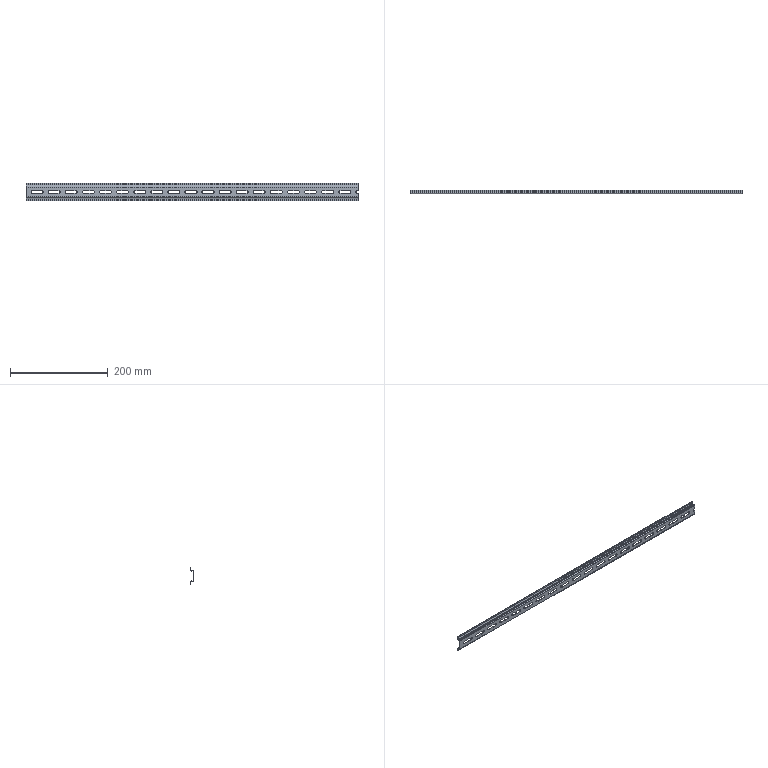Part | SolidWorks | features BaseBody 1 | 1 solid | 114 faces | box 680 x 7.5 x 35.04 mm | volume 28564 mm3 | plane 59 | cylinder 55 | commonest cylinder face diameters 5.352 x39 1.473 x8 3.473 x8